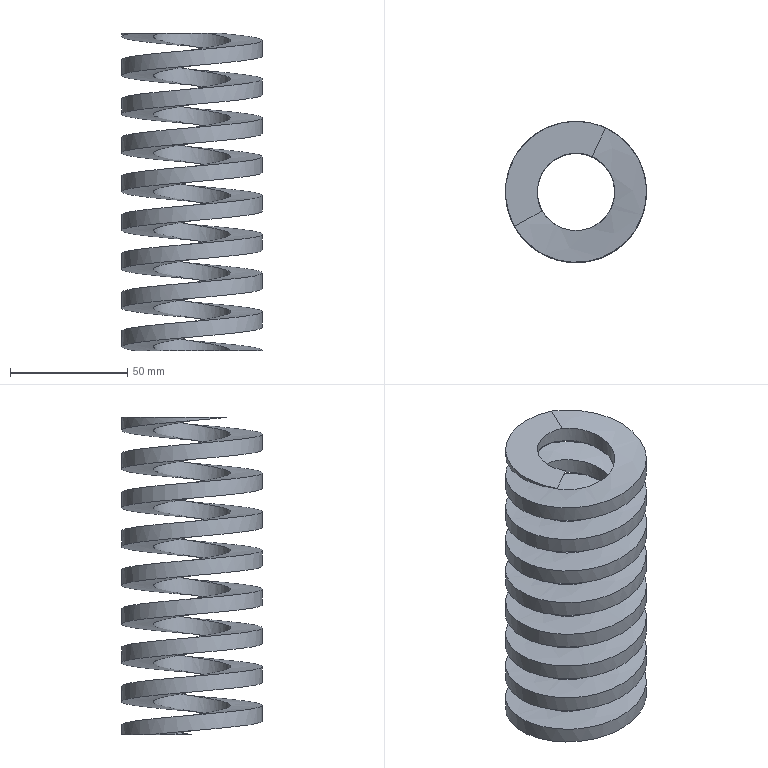Part | NX | features 模具.stp<1>[79] 2 | 1 solid | 5 faces | box 60.001 x 60 x 135.006 mm | volume 133705 mm3 | spline 2 | plane 2 | cylinder 1 | commonest cylinder face diameters 60 x1